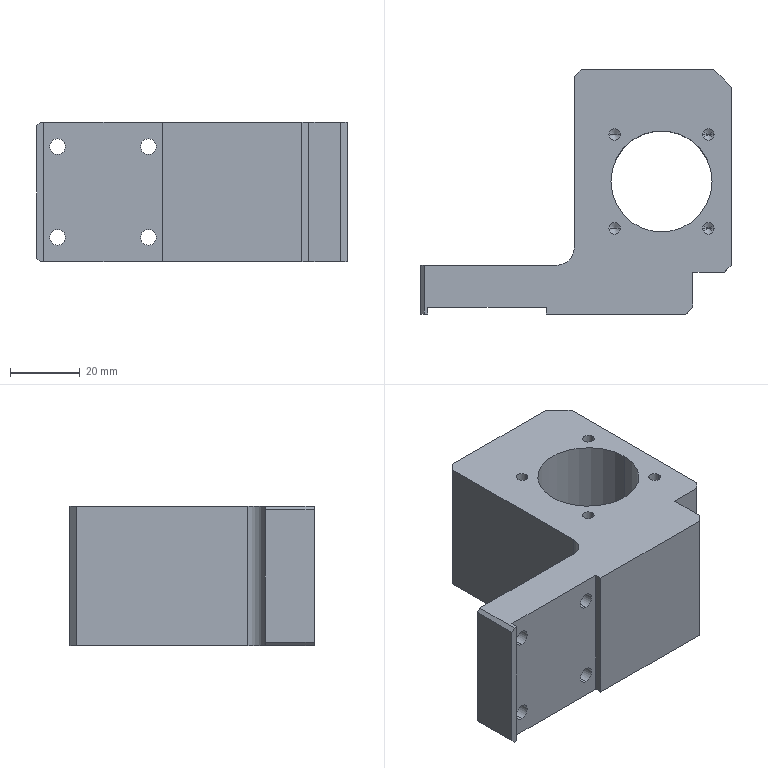Part | SolidWorks | features HoleWzd 5, Chamfer 3, ICE 3, Extrusion 1, Fillet 1 | 1 solid | 87 faces | box 89 x 70 x 40 mm | volume 113101 mm3 | cylinder 41 | plane 24 | cone 22 | commonest cylinder face diameters 3.3 x8 4.5 x8 8 x8 2.5 x6 4 x4 4.2 x4